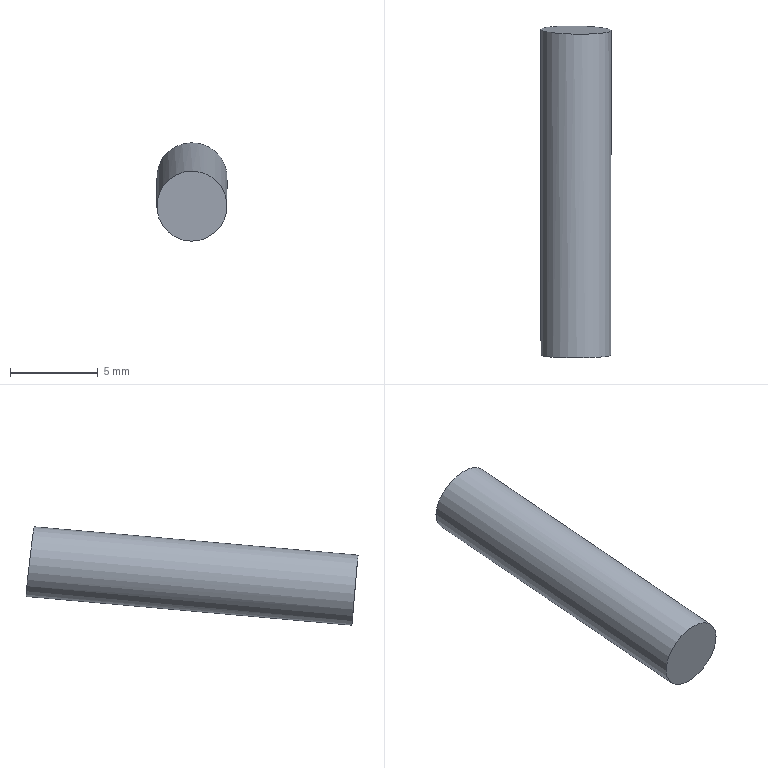Part | NX | features solid 2 | 1 solid | 3 faces | box 4 x 18.884 x 5.596 mm | volume 233.055 mm3 | plane 2 | cylinder 1 | commonest cylinder face diameters 4 x1
STEP:
#1=CARTESIAN_POINT('',(128.665,38.006,-23.445));
#2=VERTEX_POINT('',#1);
#3=CARTESIAN_POINT('',(128.148,38.174,-25.369));
#4=DIRECTION('',(0.,-0.9962,-0.08716));
#5=DIRECTION('',(0.2588,-0.08419,0.9623));
#6=AXIS2_PLACEMENT_3D('',#3,#4,#5);
#7=CIRCLE('',#6,2.);
#8=EDGE_CURVE('',#2,#2,#7,.T.);
#9=ORIENTED_EDGE('',*,*,#8,.T.);
#10=EDGE_LOOP('',(#9));
#11=FACE_BOUND('',#10,.T.);
#12=CARTESIAN_POINT('',(128.148,38.174,-25.369));
#13=DIRECTION('',(0.,-0.9962,-0.08716));
#14=DIRECTION('',(-0.2588,0.08419,-0.9623));
#15=AXIS2_PLACEMENT_3D('',#12,#13,#14);
#16=PLANE('',#15);
#17=ADVANCED_FACE('',(#11),#16,.T.);
#18=CARTESIAN_POINT('',(129.089,56.43,-22.001));
#19=VERTEX_POINT('',#18);
#20=CARTESIAN_POINT('',(128.148,56.649,-23.753));
#21=DIRECTION('',(0.01549,0.9931,0.116));
#22=DIRECTION('',(0.4705,-0.1096,0.8755));
#23=AXIS2_PLACEMENT_3D('',#20,#21,#22);
#24=ELLIPSE('',#23,2.001,2.);
#25=EDGE_CURVE('',#19,#19,#24,.T.);
#26=ORIENTED_EDGE('',*,*,#25,.T.);
#27=EDGE_LOOP('',(#26));
#28=FACE_BOUND('',#27,.T.);
#29=CARTESIAN_POINT('',(159.246,62.921,-81.584));
#30=DIRECTION('',(0.01549,0.9931,0.116));
#31=DIRECTION('',(0.06594,-0.1168,0.991));
#32=AXIS2_PLACEMENT_3D('',#29,#30,#31);
#33=PLANE('',#32);
#34=ADVANCED_FACE('',(#28),#33,.T.);
#35=ORIENTED_EDGE('',*,*,#8,.F.);
#36=EDGE_LOOP('',(#35));
#37=FACE_BOUND('',#36,.T.);
#38=ORIENTED_EDGE('',*,*,#25,.F.);
#39=EDGE_LOOP('',(#38));
#40=FACE_BOUND('',#39,.T.);
#41=CARTESIAN_POINT('',(128.148,58.098,-23.626));
#42=DIRECTION('',(0.,-0.9962,-0.08716));
#43=DIRECTION('',(-0.2588,0.08419,-0.9623));
#44=AXIS2_PLACEMENT_3D('',#41,#42,#43);
#45=CYLINDRICAL_SURFACE('',#44,2.);
#46=ADVANCED_FACE('',(#37,#40),#45,.T.);
#47=CLOSED_SHELL('',(#17,#34,#46));
#48=MANIFOLD_SOLID_BREP('',#47);
#49=(LENGTH_UNIT()NAMED_UNIT(*)SI_UNIT(.MILLI.,.METRE.));
#50=UNCERTAINTY_MEASURE_WITH_UNIT(LENGTH_MEASURE(0.00001),#49,'','');
#51=(NAMED_UNIT(*)PLANE_ANGLE_UNIT()SI_UNIT($,.RADIAN.));
#52=(NAMED_UNIT(*)SI_UNIT($,.STERADIAN.)SOLID_ANGLE_UNIT());
#53=(GEOMETRIC_REPRESENTATION_CONTEXT(3)GLOBAL_UNCERTAINTY_ASSIGNED_CONTEXT((#50))GLOBAL_UNIT_ASSIGNED_CONTEXT((#49,#51,#52))REPRESENTATION_CONTEXT('',''));
#54=ADVANCED_BREP_SHAPE_REPRESENTATION('',(#48),#53);